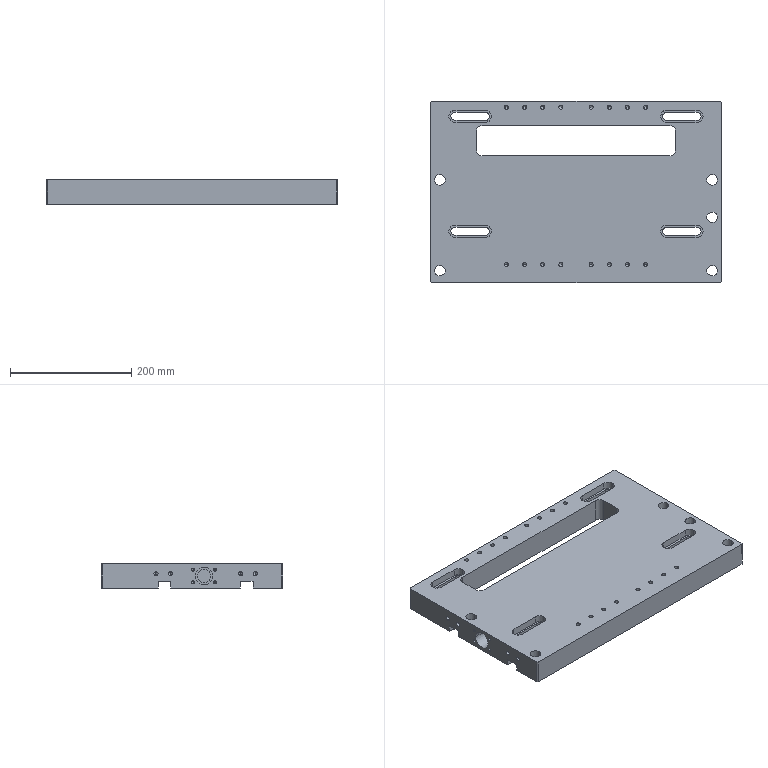Part | SolidWorks | features HoleWzd 6, ICE 6, Chamfer 1, Extrusion 1, MirrorPattern 1 | 1 solid | 225 faces | box 480 x 300 x 40 mm | volume 4575691 mm3 | cylinder 114 | cone 62 | plane 49 | commonest cylinder face diameters 6.8 x48 20 x16 13.5 x12 17.5 x10 26 x10 5 x8